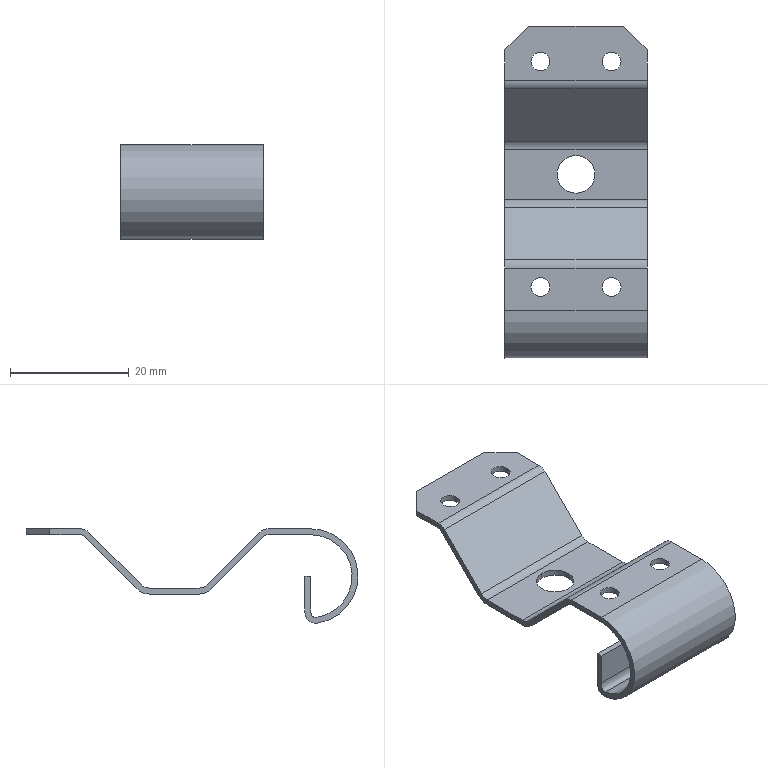Part | SolidWorks | features BaseBody 1 | 1 solid | 43 faces | box 24 x 56 x 15.934 mm | volume 1977 mm3 | cylinder 21 | plane 20 | spline 2 | commonest cylinder face diameters 3.2 x8 4 x5 2 x2 6 x2 6.35 x2 14 x1
STEP:
#1=CARTESIAN_POINT('',(4.4,-44.,0.));
#2=VERTEX_POINT('',#1);
#3=CARTESIAN_POINT('',(7.6,-44.,0.));
#4=VERTEX_POINT('',#3);
#5=CARTESIAN_POINT('',(6.,-44.,0.));
#6=DIRECTION('',(0.,0.,1.));
#7=DIRECTION('',(-1.,0.,0.));
#8=AXIS2_PLACEMENT_3D('',#5,#6,#7);
#9=CIRCLE('',#8,1.6);
#10=EDGE_CURVE('',#2,#4,#9,.T.);
#11=ORIENTED_EDGE('',*,*,#10,.T.);
#12=CARTESIAN_POINT('',(7.6,-44.,-1.));
#13=VERTEX_POINT('',#12);
#14=CARTESIAN_POINT('',(7.6,-44.,0.));
#15=DIRECTION('',(0.,0.,-1.));
#16=VECTOR('',#15,1000.);
#17=LINE('',#14,#16);
#18=EDGE_CURVE('',#4,#13,#17,.T.);
#19=ORIENTED_EDGE('',*,*,#18,.T.);
#20=CARTESIAN_POINT('',(4.4,-44.,-1.));
#21=VERTEX_POINT('',#20);
#22=CARTESIAN_POINT('',(6.,-44.,-1.));
#23=DIRECTION('',(0.,0.,-1.));
#24=DIRECTION('',(-1.,0.,0.));
#25=AXIS2_PLACEMENT_3D('',#22,#23,#24);
#26=CIRCLE('',#25,1.6);
#27=EDGE_CURVE('',#13,#21,#26,.T.);
#28=ORIENTED_EDGE('',*,*,#27,.T.);
#29=CARTESIAN_POINT('',(4.4,-44.,0.));
#30=DIRECTION('',(0.,0.,-1.));
#31=VECTOR('',#30,1000.);
#32=LINE('',#29,#31);
#33=EDGE_CURVE('',#2,#21,#32,.T.);
#34=ORIENTED_EDGE('',*,*,#33,.F.);
#35=EDGE_LOOP('',(#11,#19,#28,#34));
#36=FACE_OUTER_BOUND('',#35,.T.);
#37=CARTESIAN_POINT('',(6.,-44.,0.));
#38=DIRECTION('',(0.,0.,-1.));
#39=DIRECTION('',(-1.,0.,0.));
#40=AXIS2_PLACEMENT_3D('',#37,#38,#39);
#41=CYLINDRICAL_SURFACE('',#40,1.6);
#42=ADVANCED_FACE('',(#36),#41,.F.);
#43=CARTESIAN_POINT('',(16.4,-44.,0.));
#44=VERTEX_POINT('',#43);
#45=CARTESIAN_POINT('',(19.6,-44.,0.));
#46=VERTEX_POINT('',#45);
#47=CARTESIAN_POINT('',(18.,-44.,0.));
#48=DIRECTION('',(0.,0.,1.));
#49=DIRECTION('',(-1.,0.,0.));
#50=AXIS2_PLACEMENT_3D('',#47,#48,#49);
#51=CIRCLE('',#50,1.6);
#52=EDGE_CURVE('',#44,#46,#51,.T.);
#53=ORIENTED_EDGE('',*,*,#52,.T.);
#54=CARTESIAN_POINT('',(19.6,-44.,-1.));
#55=VERTEX_POINT('',#54);
#56=CARTESIAN_POINT('',(19.6,-44.,0.));
#57=DIRECTION('',(0.,0.,-1.));
#58=VECTOR('',#57,1000.);
#59=LINE('',#56,#58);
#60=EDGE_CURVE('',#46,#55,#59,.T.);
#61=ORIENTED_EDGE('',*,*,#60,.T.);
#62=CARTESIAN_POINT('',(16.4,-44.,-1.));
#63=VERTEX_POINT('',#62);
#64=CARTESIAN_POINT('',(18.,-44.,-1.));
#65=DIRECTION('',(0.,0.,-1.));
#66=DIRECTION('',(-1.,0.,0.));
#67=AXIS2_PLACEMENT_3D('',#64,#65,#66);
#68=CIRCLE('',#67,1.6);
#69=EDGE_CURVE('',#55,#63,#68,.T.);
#70=ORIENTED_EDGE('',*,*,#69,.T.);
#71=CARTESIAN_POINT('',(16.4,-44.,0.));
#72=DIRECTION('',(0.,0.,-1.));
#73=VECTOR('',#72,1000.);
#74=LINE('',#71,#73);
#75=EDGE_CURVE('',#44,#63,#74,.T.);
#76=ORIENTED_EDGE('',*,*,#75,.F.);
#77=EDGE_LOOP('',(#53,#61,#70,#76));
#78=FACE_OUTER_BOUND('',#77,.T.);
#79=CARTESIAN_POINT('',(18.,-44.,0.));
#80=DIRECTION('',(0.,0.,-1.));
#81=DIRECTION('',(-1.,0.,0.));
#82=AXIS2_PLACEMENT_3D('',#79,#80,#81);
#83=CYLINDRICAL_SURFACE('',#82,1.6);
#84=ADVANCED_FACE('',(#78),#83,.F.);
#85=CARTESIAN_POINT('',(16.4,-6.,0.));
#86=VERTEX_POINT('',#85);
#87=CARTESIAN_POINT('',(19.6,-6.,0.));
#88=VERTEX_POINT('',#87);
#89=CARTESIAN_POINT('',(18.,-6.,0.));
#90=DIRECTION('',(0.,0.,1.));
#91=DIRECTION('',(-1.,0.,0.));
#92=AXIS2_PLACEMENT_3D('',#89,#90,#91);
#93=CIRCLE('',#92,1.6);
#94=EDGE_CURVE('',#86,#88,#93,.T.);
#95=ORIENTED_EDGE('',*,*,#94,.T.);
#96=CARTESIAN_POINT('',(19.6,-6.,-1.));
#97=VERTEX_POINT('',#96);
#98=CARTESIAN_POINT('',(19.6,-6.,0.));
#99=DIRECTION('',(0.,0.,-1.));
#100=VECTOR('',#99,1000.);
#101=LINE('',#98,#100);
#102=EDGE_CURVE('',#88,#97,#101,.T.);
#103=ORIENTED_EDGE('',*,*,#102,.T.);
#104=CARTESIAN_POINT('',(16.4,-6.,-1.));
#105=VERTEX_POINT('',#104);
#106=CARTESIAN_POINT('',(18.,-6.,-1.));
#107=DIRECTION('',(0.,0.,-1.));
#108=DIRECTION('',(-1.,0.,0.));
#109=AXIS2_PLACEMENT_3D('',#106,#107,#108);
#110=CIRCLE('',#109,1.6);
#111=EDGE_CURVE('',#97,#105,#110,.T.);
#112=ORIENTED_EDGE('',*,*,#111,.T.);
#113=CARTESIAN_POINT('',(16.4,-6.,0.));
#114=DIRECTION('',(0.,0.,-1.));
#115=VECTOR('',#114,1000.);
#116=LINE('',#113,#115);
#117=EDGE_CURVE('',#86,#105,#116,.T.);
#118=ORIENTED_EDGE('',*,*,#117,.F.);
#119=EDGE_LOOP('',(#95,#103,#112,#118));
#120=FACE_OUTER_BOUND('',#119,.T.);
#121=CARTESIAN_POINT('',(18.,-6.,0.));
#122=DIRECTION('',(0.,0.,-1.));
#123=DIRECTION('',(-1.,0.,0.));
#124=AXIS2_PLACEMENT_3D('',#121,#122,#123);
#125=CYLINDRICAL_SURFACE('',#124,1.6);
#126=ADVANCED_FACE('',(#120),#125,.F.);
#127=CARTESIAN_POINT('',(4.4,-6.,0.));
#128=VERTEX_POINT('',#127);
#129=CARTESIAN_POINT('',(7.6,-6.,0.));
#130=VERTEX_POINT('',#129);
#131=CARTESIAN_POINT('',(6.,-6.,0.));
#132=DIRECTION('',(0.,0.,1.));
#133=DIRECTION('',(-1.,0.,0.));
#134=AXIS2_PLACEMENT_3D('',#131,#132,#133);
#135=CIRCLE('',#134,1.6);
#136=EDGE_CURVE('',#128,#130,#135,.T.);
#137=ORIENTED_EDGE('',*,*,#136,.T.);
#138=CARTESIAN_POINT('',(7.6,-6.,-1.));
#139=VERTEX_POINT('',#138);
#140=CARTESIAN_POINT('',(7.6,-6.,0.));
#141=DIRECTION('',(0.,0.,-1.));
#142=VECTOR('',#141,1000.);
#143=LINE('',#140,#142);
#144=EDGE_CURVE('',#130,#139,#143,.T.);
#145=ORIENTED_EDGE('',*,*,#144,.T.);
#146=CARTESIAN_POINT('',(4.4,-6.,-1.));
#147=VERTEX_POINT('',#146);
#148=CARTESIAN_POINT('',(6.,-6.,-1.));
#149=DIRECTION('',(0.,0.,-1.));
#150=DIRECTION('',(-1.,0.,0.));
#151=AXIS2_PLACEMENT_3D('',#148,#149,#150);
#152=CIRCLE('',#151,1.6);
#153=EDGE_CURVE('',#139,#147,#152,.T.);
#154=ORIENTED_EDGE('',*,*,#153,.T.);
#155=CARTESIAN_POINT('',(4.4,-6.,0.));
#156=DIRECTION('',(0.,0.,-1.));
#157=VECTOR('',#156,1000.);
#158=LINE('',#155,#157);
#159=EDGE_CURVE('',#128,#147,#158,.T.);
#160=ORIENTED_EDGE('',*,*,#159,.F.);
#161=EDGE_LOOP('',(#137,#145,#154,#160));
#162=FACE_OUTER_BOUND('',#161,.T.);
#163=CARTESIAN_POINT('',(6.,-6.,0.));
#164=DIRECTION('',(0.,0.,-1.));
#165=DIRECTION('',(-1.,0.,0.));
#166=AXIS2_PLACEMENT_3D('',#163,#164,#165);
#167=CYLINDRICAL_SURFACE('',#166,1.6);
#168=ADVANCED_FACE('',(#162),#167,.F.);
#169=CARTESIAN_POINT('',(12.,-21.825,-10.));
#170=VERTEX_POINT('',#169);
#171=CARTESIAN_POINT('',(12.,-28.175,-10.));
#172=VERTEX_POINT('',#171);
#173=CARTESIAN_POINT('',(12.,-25.,-10.));
#174=DIRECTION('',(0.,0.,1.));
#175=DIRECTION('',(0.,1.,0.));
#176=AXIS2_PLACEMENT_3D('',#173,#174,#175);
#177=CIRCLE('',#176,3.175);
#178=EDGE_CURVE('',#170,#172,#177,.T.);
#179=ORIENTED_EDGE('',*,*,#178,.T.);
#180=CARTESIAN_POINT('',(12.,-28.175,-11.));
#181=VERTEX_POINT('',#180);
#182=CARTESIAN_POINT('',(12.,-28.175,-10.));
#183=DIRECTION('',(0.,0.,-1.));
#184=VECTOR('',#183,1000.);
#185=LINE('',#182,#184);
#186=EDGE_CURVE('',#172,#181,#185,.T.);
#187=ORIENTED_EDGE('',*,*,#186,.T.);
#188=CARTESIAN_POINT('',(12.,-21.825,-11.));
#189=VERTEX_POINT('',#188);
#190=CARTESIAN_POINT('',(12.,-25.,-11.));
#191=DIRECTION('',(0.,0.,-1.));
#192=DIRECTION('',(0.,1.,0.));
#193=AXIS2_PLACEMENT_3D('',#190,#191,#192);
#194=CIRCLE('',#193,3.175);
#195=EDGE_CURVE('',#181,#189,#194,.T.);
#196=ORIENTED_EDGE('',*,*,#195,.T.);
#197=CARTESIAN_POINT('',(12.,-21.825,-10.));
#198=DIRECTION('',(0.,0.,-1.));
#199=VECTOR('',#198,1000.);
#200=LINE('',#197,#199);
#201=EDGE_CURVE('',#170,#189,#200,.T.);
#202=ORIENTED_EDGE('',*,*,#201,.F.);
#203=EDGE_LOOP('',(#179,#187,#196,#202));
#204=FACE_OUTER_BOUND('',#203,.T.);
#205=CARTESIAN_POINT('',(12.,-25.,-10.));
#206=DIRECTION('',(0.,0.,-1.));
#207=DIRECTION('',(0.,1.,0.));
#208=AXIS2_PLACEMENT_3D('',#205,#206,#207);
#209=CYLINDRICAL_SURFACE('',#208,3.175);
#210=ADVANCED_FACE('',(#204),#209,.F.);
#211=ORIENTED_EDGE('',*,*,#18,.F.);
#212=CARTESIAN_POINT('',(6.,-44.,0.));
#213=DIRECTION('',(0.,0.,1.));
#214=DIRECTION('',(-1.,0.,0.));
#215=AXIS2_PLACEMENT_3D('',#212,#213,#214);
#216=CIRCLE('',#215,1.6);
#217=EDGE_CURVE('',#4,#2,#216,.T.);
#218=ORIENTED_EDGE('',*,*,#217,.T.);
#219=ORIENTED_EDGE('',*,*,#33,.T.);
#220=CARTESIAN_POINT('',(6.,-44.,-1.));
#221=DIRECTION('',(0.,0.,-1.));
#222=DIRECTION('',(-1.,0.,0.));
#223=AXIS2_PLACEMENT_3D('',#220,#221,#222);
#224=CIRCLE('',#223,1.6);
#225=EDGE_CURVE('',#21,#13,#224,.T.);
#226=ORIENTED_EDGE('',*,*,#225,.T.);
#227=EDGE_LOOP('',(#211,#218,#219,#226));
#228=FACE_OUTER_BOUND('',#227,.T.);
#229=CARTESIAN_POINT('',(6.,-44.,0.));
#230=DIRECTION('',(0.,0.,-1.));
#231=DIRECTION('',(-1.,0.,0.));
#232=AXIS2_PLACEMENT_3D('',#229,#230,#231);
#233=CYLINDRICAL_SURFACE('',#232,1.6);
#234=ADVANCED_FACE('',(#228),#233,.F.);
#235=CARTESIAN_POINT('',(18.,-44.,-1.));
#236=DIRECTION('',(0.,0.,-1.));
#237=DIRECTION('',(-1.,0.,0.));
#238=AXIS2_PLACEMENT_3D('',#235,#236,#237);
#239=CIRCLE('',#238,1.6);
#240=EDGE_CURVE('',#63,#55,#239,.T.);
#241=ORIENTED_EDGE('',*,*,#240,.F.);
#242=ORIENTED_EDGE('',*,*,#69,.F.);
#243=EDGE_LOOP('',(#241,#242));
#244=FACE_BOUND('',#243,.T.);
#245=ORIENTED_EDGE('',*,*,#225,.F.);
#246=ORIENTED_EDGE('',*,*,#27,.F.);
#247=EDGE_LOOP('',(#245,#246));
#248=FACE_BOUND('',#247,.T.);
#249=CARTESIAN_POINT('',(24.,-40.828,-1.));
#250=VERTEX_POINT('',#249);
#251=CARTESIAN_POINT('',(0.,-40.828,-1.));
#252=VERTEX_POINT('',#251);
#253=CARTESIAN_POINT('',(12.,-40.828,-1.));
#254=DIRECTION('',(-1.,0.,0.));
#255=VECTOR('',#254,1000.);
#256=LINE('',#253,#255);
#257=EDGE_CURVE('',#250,#252,#256,.T.);
#258=ORIENTED_EDGE('',*,*,#257,.F.);
#259=CARTESIAN_POINT('',(24.,-48.,-1.));
#260=VERTEX_POINT('',#259);
#261=CARTESIAN_POINT('',(24.,-44.414,-1.));
#262=DIRECTION('',(0.,1.,0.));
#263=VECTOR('',#262,1000.);
#264=LINE('',#261,#263);
#265=EDGE_CURVE('',#260,#250,#264,.T.);
#266=ORIENTED_EDGE('',*,*,#265,.F.);
#267=CARTESIAN_POINT('',(0.,-48.,-1.));
#268=VERTEX_POINT('',#267);
#269=CARTESIAN_POINT('',(12.,-48.,-1.));
#270=DIRECTION('',(1.,0.,0.));
#271=VECTOR('',#270,1000.);
#272=LINE('',#269,#271);
#273=EDGE_CURVE('',#268,#260,#272,.T.);
#274=ORIENTED_EDGE('',*,*,#273,.F.);
#275=CARTESIAN_POINT('',(0.,-44.414,-1.));
#276=DIRECTION('',(0.,-1.,0.));
#277=VECTOR('',#276,1000.);
#278=LINE('',#275,#277);
#279=EDGE_CURVE('',#252,#268,#278,.T.);
#280=ORIENTED_EDGE('',*,*,#279,.F.);
#281=EDGE_LOOP('',(#258,#266,#274,#280));
#282=FACE_OUTER_BOUND('',#281,.T.);
#283=CARTESIAN_POINT('',(0.,-40.828,-1.));
#284=DIRECTION('',(0.,0.,1.));
#285=DIRECTION('',(0.,-1.,0.));
#286=AXIS2_PLACEMENT_3D('',#283,#284,#285);
#287=PLANE('',#286);
#288=ADVANCED_FACE('',(#244,#248,#282),#287,.F.);
#289=ORIENTED_EDGE('',*,*,#52,.F.);
#290=CARTESIAN_POINT('',(18.,-44.,0.));
#291=DIRECTION('',(0.,0.,1.));
#292=DIRECTION('',(-1.,0.,0.));
#293=AXIS2_PLACEMENT_3D('',#290,#291,#292);
#294=CIRCLE('',#293,1.6);
#295=EDGE_CURVE('',#46,#44,#294,.T.);
#296=ORIENTED_EDGE('',*,*,#295,.F.);
#297=EDGE_LOOP('',(#289,#296));
#298=FACE_BOUND('',#297,.T.);
#299=ORIENTED_EDGE('',*,*,#10,.F.);
#300=ORIENTED_EDGE('',*,*,#217,.F.);
#301=EDGE_LOOP('',(#299,#300));
#302=FACE_BOUND('',#301,.T.);
#303=CARTESIAN_POINT('',(24.,-48.,0.));
#304=VERTEX_POINT('',#303);
#305=CARTESIAN_POINT('',(0.,-48.,0.));
#306=VERTEX_POINT('',#305);
#307=CARTESIAN_POINT('',(12.,-48.,0.));
#308=DIRECTION('',(-1.,0.,0.));
#309=VECTOR('',#308,1000.);
#310=LINE('',#307,#309);
#311=EDGE_CURVE('',#304,#306,#310,.T.);
#312=ORIENTED_EDGE('',*,*,#311,.F.);
#313=CARTESIAN_POINT('',(24.,-40.828,0.));
#314=VERTEX_POINT('',#313);
#315=CARTESIAN_POINT('',(24.,-44.414,0.));
#316=DIRECTION('',(0.,-1.,0.));
#317=VECTOR('',#316,1000.);
#318=LINE('',#315,#317);
#319=EDGE_CURVE('',#314,#304,#318,.T.);
#320=ORIENTED_EDGE('',*,*,#319,.F.);
#321=CARTESIAN_POINT('',(0.,-40.828,0.));
#322=VERTEX_POINT('',#321);
#323=CARTESIAN_POINT('',(12.,-40.828,0.));
#324=DIRECTION('',(1.,0.,0.));
#325=VECTOR('',#324,1000.);
#326=LINE('',#323,#325);
#327=EDGE_CURVE('',#322,#314,#326,.T.);
#328=ORIENTED_EDGE('',*,*,#327,.F.);
#329=CARTESIAN_POINT('',(0.,-44.414,0.));
#330=DIRECTION('',(0.,1.,0.));
#331=VECTOR('',#330,1000.);
#332=LINE('',#329,#331);
#333=EDGE_CURVE('',#306,#322,#332,.T.);
#334=ORIENTED_EDGE('',*,*,#333,.F.);
#335=EDGE_LOOP('',(#312,#320,#328,#334));
#336=FACE_OUTER_BOUND('',#335,.T.);
#337=CARTESIAN_POINT('',(0.,-48.,0.));
#338=DIRECTION('',(0.,0.,-1.));
#339=DIRECTION('',(0.,1.,0.));
#340=AXIS2_PLACEMENT_3D('',#337,#338,#339);
#341=PLANE('',#340);
#342=ADVANCED_FACE('',(#298,#302,#336),#341,.F.);
#343=ORIENTED_EDGE('',*,*,#60,.F.);
#344=ORIENTED_EDGE('',*,*,#295,.T.);
#345=ORIENTED_EDGE('',*,*,#75,.T.);
#346=ORIENTED_EDGE('',*,*,#240,.T.);
#347=EDGE_LOOP('',(#343,#344,#345,#346));
#348=FACE_OUTER_BOUND('',#347,.T.);
#349=CARTESIAN_POINT('',(18.,-44.,0.));
#350=DIRECTION('',(0.,0.,-1.));
#351=DIRECTION('',(-1.,0.,0.));
#352=AXIS2_PLACEMENT_3D('',#349,#350,#351);
#353=CYLINDRICAL_SURFACE('',#352,1.6);
#354=ADVANCED_FACE('',(#348),#353,.F.);
#355=CARTESIAN_POINT('',(0.,-4.,0.));
#356=VERTEX_POINT('',#355);
#357=CARTESIAN_POINT('',(0.,-4.,-1.));
#358=VERTEX_POINT('',#357);
#359=CARTESIAN_POINT('',(0.,-4.,-0.5));
#360=DIRECTION('',(0.,0.,-1.));
#361=VECTOR('',#360,1000.);
#362=LINE('',#359,#361);
#363=EDGE_CURVE('',#356,#358,#362,.T.);
#364=ORIENTED_EDGE('',*,*,#363,.T.);
#365=CARTESIAN_POINT('',(0.,-9.172,-1.));
#366=VERTEX_POINT('',#365);
#367=CARTESIAN_POINT('',(0.,-30.156,-1.));
#368=DIRECTION('',(0.,1.,0.));
#369=VECTOR('',#368,1000.);
#370=LINE('',#367,#369);
#371=EDGE_CURVE('',#366,#358,#370,.T.);
#372=ORIENTED_EDGE('',*,*,#371,.F.);
#373=CARTESIAN_POINT('',(0.,-9.879,-1.293));
#374=VERTEX_POINT('',#373);
#375=CARTESIAN_POINT('',(0.,-9.172,-2.));
#376=DIRECTION('',(-1.,0.,0.));
#377=DIRECTION('',(0.,0.,1.));
#378=AXIS2_PLACEMENT_3D('',#375,#376,#377);
#379=CIRCLE('',#378,1.);
#380=EDGE_CURVE('',#374,#366,#379,.T.);
#381=ORIENTED_EDGE('',*,*,#380,.F.);
#382=CARTESIAN_POINT('',(0.,-18.707,-10.121));
#383=VERTEX_POINT('',#382);
#384=CARTESIAN_POINT('',(0.,-9.879,-1.293));
#385=DIRECTION('',(0.,0.7071,0.7071));
#386=VECTOR('',#385,1000.);
#387=LINE('',#384,#386);
#388=EDGE_CURVE('',#383,#374,#387,.T.);
#389=ORIENTED_EDGE('',*,*,#388,.F.);
#390=CARTESIAN_POINT('',(0.,-20.828,-11.));
#391=VERTEX_POINT('',#390);
#392=CARTESIAN_POINT('',(0.,-20.828,-8.));
#393=DIRECTION('',(1.,0.,0.));
#394=DIRECTION('',(0.,0.,1.));
#395=AXIS2_PLACEMENT_3D('',#392,#393,#394);
#396=CIRCLE('',#395,3.);
#397=EDGE_CURVE('',#391,#383,#396,.T.);
#398=ORIENTED_EDGE('',*,*,#397,.F.);
#399=CARTESIAN_POINT('',(0.,-29.172,-11.));
#400=VERTEX_POINT('',#399);
#401=CARTESIAN_POINT('',(0.,-30.156,-11.));
#402=DIRECTION('',(0.,1.,0.));
#403=VECTOR('',#402,1000.);
#404=LINE('',#401,#403);
#405=EDGE_CURVE('',#400,#391,#404,.T.);
#406=ORIENTED_EDGE('',*,*,#405,.F.);
#407=CARTESIAN_POINT('',(0.,-31.293,-10.121));
#408=VERTEX_POINT('',#407);
#409=CARTESIAN_POINT('',(0.,-29.172,-8.));
#410=DIRECTION('',(1.,0.,0.));
#411=DIRECTION('',(0.,0.,1.));
#412=AXIS2_PLACEMENT_3D('',#409,#410,#411);
#413=CIRCLE('',#412,3.);
#414=EDGE_CURVE('',#408,#400,#413,.T.);
#415=ORIENTED_EDGE('',*,*,#414,.F.);
#416=CARTESIAN_POINT('',(0.,-40.121,-1.293));
#417=VERTEX_POINT('',#416);
#418=CARTESIAN_POINT('',(0.,-31.293,-10.121));
#419=DIRECTION('',(0.,0.7071,-0.7071));
#420=VECTOR('',#419,1000.);
#421=LINE('',#418,#420);
#422=EDGE_CURVE('',#417,#408,#421,.T.);
#423=ORIENTED_EDGE('',*,*,#422,.F.);
#424=CARTESIAN_POINT('',(0.,-40.828,-2.));
#425=DIRECTION('',(-1.,0.,0.));
#426=DIRECTION('',(0.,0.,1.));
#427=AXIS2_PLACEMENT_3D('',#424,#425,#426);
#428=CIRCLE('',#427,1.);
#429=EDGE_CURVE('',#252,#417,#428,.T.);
#430=ORIENTED_EDGE('',*,*,#429,.F.);
#431=ORIENTED_EDGE('',*,*,#279,.T.);
#432=CARTESIAN_POINT('',(0.,-49.061,-14.919));
#433=VERTEX_POINT('',#432);
#434=CARTESIAN_POINT('',(0.,-48.,-8.));
#435=DIRECTION('',(-1.,0.,0.));
#436=DIRECTION('',(0.,0.,1.));
#437=AXIS2_PLACEMENT_3D('',#434,#435,#436);
#438=CIRCLE('',#437,7.);
#439=EDGE_CURVE('',#433,#268,#438,.T.);
#440=ORIENTED_EDGE('',*,*,#439,.F.);
#441=CARTESIAN_POINT('',(0.,-48.,-13.525));
#442=VERTEX_POINT('',#441);
#443=CARTESIAN_POINT('',(0.,-48.,-13.525));
#444=CARTESIAN_POINT('',(0.,-48.,-13.685));
#445=CARTESIAN_POINT('',(0.,-48.019,-14.03));
#446=CARTESIAN_POINT('',(0.,-48.12,-14.503));
#447=CARTESIAN_POINT('',(0.,-48.264,-14.743));
#448=CARTESIAN_POINT('',(0.,-48.382,-14.839));
#449=CARTESIAN_POINT('',(0.,-48.506,-14.898));
#450=CARTESIAN_POINT('',(0.,-48.706,-14.941));
#451=CARTESIAN_POINT('',(0.,-48.953,-14.932));
#452=CARTESIAN_POINT('',(0.,-49.061,-14.919));
#453=B_SPLINE_CURVE_WITH_KNOTS('',3,(#443,#444,#445,#446,#447,#448,#449,#450,#451,#452),.UNSPECIFIED.,.F.,.F.,(4,1,1,1,1,1,1,4),(0.,0.0002613,0.0005226,0.001045,0.001306,0.001568,0.001829,0.00209),.UNSPECIFIED.);
#454=EDGE_CURVE('',#442,#433,#453,.T.);
#455=ORIENTED_EDGE('',*,*,#454,.F.);
#456=CARTESIAN_POINT('',(0.,-48.,-8.011));
#457=VERTEX_POINT('',#456);
#458=CARTESIAN_POINT('',(0.,-48.,-8.021));
#459=DIRECTION('',(0.,0.,-1.));
#460=VECTOR('',#459,1000.);
#461=LINE('',#458,#460);
#462=EDGE_CURVE('',#457,#442,#461,.T.);
#463=ORIENTED_EDGE('',*,*,#462,.F.);
#464=CARTESIAN_POINT('',(0.,-47.,-8.011));
#465=VERTEX_POINT('',#464);
#466=CARTESIAN_POINT('',(0.,-47.5,-8.011));
#467=DIRECTION('',(0.,1.,0.));
#468=VECTOR('',#467,1000.);
#469=LINE('',#466,#468);
#470=EDGE_CURVE('',#457,#465,#469,.T.);
#471=ORIENTED_EDGE('',*,*,#470,.T.);
#472=CARTESIAN_POINT('',(0.,-47.,-13.525));
#473=VERTEX_POINT('',#472);
#474=CARTESIAN_POINT('',(0.,-47.,-8.021));
#475=DIRECTION('',(0.,0.,1.));
#476=VECTOR('',#475,1000.);
#477=LINE('',#474,#476);
#478=EDGE_CURVE('',#473,#465,#477,.T.);
#479=ORIENTED_EDGE('',*,*,#478,.F.);
#480=CARTESIAN_POINT('',(0.,-49.198,-15.91));
#481=VERTEX_POINT('',#480);
#482=CARTESIAN_POINT('',(0.,-49.198,-15.91));
#483=CARTESIAN_POINT('',(0.,-47.739,-16.093));
#484=CARTESIAN_POINT('',(0.,-47.,-15.237));
#485=CARTESIAN_POINT('',(0.,-47.,-13.525));
#486=B_SPLINE_CURVE_WITH_KNOTS('',3,(#482,#483,#484,#485),.UNSPECIFIED.,.F.,.F.,(4,4),(0.,0.003798),.UNSPECIFIED.);
#487=EDGE_CURVE('',#481,#473,#486,.T.);
#488=ORIENTED_EDGE('',*,*,#487,.F.);
#489=CARTESIAN_POINT('',(0.,-48.,-8.));
#490=DIRECTION('',(1.,0.,0.));
#491=DIRECTION('',(0.,0.,1.));
#492=AXIS2_PLACEMENT_3D('',#489,#490,#491);
#493=CIRCLE('',#492,8.);
#494=EDGE_CURVE('',#306,#481,#493,.T.);
#495=ORIENTED_EDGE('',*,*,#494,.F.);
#496=ORIENTED_EDGE('',*,*,#333,.T.);
#497=CARTESIAN_POINT('',(0.,-39.414,-0.5858));
#498=VERTEX_POINT('',#497);
#499=CARTESIAN_POINT('',(0.,-40.828,-2.));
#500=DIRECTION('',(1.,0.,0.));
#501=DIRECTION('',(0.,0.,1.));
#502=AXIS2_PLACEMENT_3D('',#499,#500,#501);
#503=CIRCLE('',#502,2.);
#504=EDGE_CURVE('',#498,#322,#503,.T.);
#505=ORIENTED_EDGE('',*,*,#504,.F.);
#506=CARTESIAN_POINT('',(0.,-30.586,-9.414));
#507=VERTEX_POINT('',#506);
#508=CARTESIAN_POINT('',(0.,-39.414,-0.5858));
#509=DIRECTION('',(0.,-0.7071,0.7071));
#510=VECTOR('',#509,1000.);
#511=LINE('',#508,#510);
#512=EDGE_CURVE('',#507,#498,#511,.T.);
#513=ORIENTED_EDGE('',*,*,#512,.F.);
#514=CARTESIAN_POINT('',(0.,-29.172,-10.));
#515=VERTEX_POINT('',#514);
#516=CARTESIAN_POINT('',(0.,-29.172,-8.));
#517=DIRECTION('',(-1.,0.,0.));
#518=DIRECTION('',(0.,0.,1.));
#519=AXIS2_PLACEMENT_3D('',#516,#517,#518);
#520=CIRCLE('',#519,2.);
#521=EDGE_CURVE('',#515,#507,#520,.T.);
#522=ORIENTED_EDGE('',*,*,#521,.F.);
#523=CARTESIAN_POINT('',(0.,-20.828,-10.));
#524=VERTEX_POINT('',#523);
#525=CARTESIAN_POINT('',(0.,-30.156,-10.));
#526=DIRECTION('',(0.,-1.,0.));
#527=VECTOR('',#526,1000.);
#528=LINE('',#525,#527);
#529=EDGE_CURVE('',#524,#515,#528,.T.);
#530=ORIENTED_EDGE('',*,*,#529,.F.);
#531=CARTESIAN_POINT('',(0.,-19.414,-9.414));
#532=VERTEX_POINT('',#531);
#533=CARTESIAN_POINT('',(0.,-20.828,-8.));
#534=DIRECTION('',(-1.,0.,0.));
#535=DIRECTION('',(0.,0.,1.));
#536=AXIS2_PLACEMENT_3D('',#533,#534,#535);
#537=CIRCLE('',#536,2.);
#538=EDGE_CURVE('',#532,#524,#537,.T.);
#539=ORIENTED_EDGE('',*,*,#538,.F.);
#540=CARTESIAN_POINT('',(0.,-10.586,-0.5858));
#541=VERTEX_POINT('',#540);
#542=CARTESIAN_POINT('',(0.,-19.414,-9.414));
#543=DIRECTION('',(0.,-0.7071,-0.7071));
#544=VECTOR('',#543,1000.);
#545=LINE('',#542,#544);
#546=EDGE_CURVE('',#541,#532,#545,.T.);
#547=ORIENTED_EDGE('',*,*,#546,.F.);
#548=CARTESIAN_POINT('',(0.,-9.172,0.));
#549=VERTEX_POINT('',#548);
#550=CARTESIAN_POINT('',(0.,-9.172,-2.));
#551=DIRECTION('',(-1.,0.,0.));
#552=DIRECTION('',(0.,0.,1.));
#553=AXIS2_PLACEMENT_3D('',#550,#551,#552);
#554=CIRCLE('',#553,2.);
#555=EDGE_CURVE('',#541,#549,#554,.T.);
#556=ORIENTED_EDGE('',*,*,#555,.T.);
#557=CARTESIAN_POINT('',(0.,-30.156,0.));
#558=DIRECTION('',(0.,-1.,0.));
#559=VECTOR('',#558,1000.);
#560=LINE('',#557,#559);
#561=EDGE_CURVE('',#356,#549,#560,.T.);
#562=ORIENTED_EDGE('',*,*,#561,.F.);
#563=EDGE_LOOP('',(#364,#372,#381,#389,#398,#406,#415,#423,#430,#431,#440,#455,#463,#471,#479,#488,#495,#496,#505,#513,#522,#530,#539,#547,#556,#562));
#564=FACE_OUTER_BOUND('',#563,.T.);
#565=CARTESIAN_POINT('',(0.,-56.312,0.));
#566=DIRECTION('',(1.,0.,0.));
#567=DIRECTION('',(0.,0.,-1.));
#568=AXIS2_PLACEMENT_3D('',#565,#566,#567);
#569=PLANE('',#568);
#570=ADVANCED_FACE('',(#564),#569,.F.);
#571=CARTESIAN_POINT('',(24.,-40.121,-1.293));
#572=VERTEX_POINT('',#571);
#573=CARTESIAN_POINT('',(24.,-40.828,-2.));
#574=DIRECTION('',(1.,0.,0.));
#575=DIRECTION('',(0.,0.,1.));
#576=AXIS2_PLACEMENT_3D('',#573,#574,#575);
#577=CIRCLE('',#576,1.);
#578=EDGE_CURVE('',#572,#250,#577,.T.);
#579=ORIENTED_EDGE('',*,*,#578,.T.);
#580=ORIENTED_EDGE('',*,*,#257,.T.);
#581=ORIENTED_EDGE('',*,*,#429,.T.);
#582=CARTESIAN_POINT('',(12.,-40.121,-1.293));
#583=DIRECTION('',(1.,0.,0.));
#584=VECTOR('',#583,1000.);
#585=LINE('',#582,#584);
#586=EDGE_CURVE('',#417,#572,#585,.T.);
#587=ORIENTED_EDGE('',*,*,#586,.T.);
#588=EDGE_LOOP('',(#579,#580,#581,#587));
#589=FACE_OUTER_BOUND('',#588,.T.);
#590=CARTESIAN_POINT('',(24.,-40.828,-2.));
#591=DIRECTION('',(-1.,0.,0.));
#592=DIRECTION('',(0.,0.,1.));
#593=AXIS2_PLACEMENT_3D('',#590,#591,#592);
#594=CYLINDRICAL_SURFACE('',#593,1.);
#595=ADVANCED_FACE('',(#589),#594,.F.);
#596=CARTESIAN_POINT('',(24.,-49.198,-15.91));
#597=VERTEX_POINT('',#596);
#598=CARTESIAN_POINT('',(24.,-47.,-13.525));
#599=VERTEX_POINT('',#598);
#600=CARTESIAN_POINT('',(24.,-49.198,-15.91));
#601=CARTESIAN_POINT('',(24.,-47.739,-16.093));
#602=CARTESIAN_POINT('',(24.,-47.,-15.237));
#603=CARTESIAN_POINT('',(24.,-47.,-13.525));
#604=B_SPLINE_CURVE_WITH_KNOTS('',3,(#600,#601,#602,#603),.UNSPECIFIED.,.F.,.F.,(4,4),(0.,0.003798),.UNSPECIFIED.);
#605=EDGE_CURVE('',#597,#599,#604,.T.);
#606=ORIENTED_EDGE('',*,*,#605,.T.);
#607=CARTESIAN_POINT('',(24.,-47.,-11.011));
#608=VERTEX_POINT('',#607);
#609=CARTESIAN_POINT('',(24.,-47.,-8.021));
#610=DIRECTION('',(0.,0.,1.));
#611=VECTOR('',#610,1000.);
#612=LINE('',#609,#611);
#613=EDGE_CURVE('',#599,#608,#612,.T.);
#614=ORIENTED_EDGE('',*,*,#613,.T.);
#615=CARTESIAN_POINT('',(24.,-48.,-11.011));
#616=VERTEX_POINT('',#615);
#617=CARTESIAN_POINT('',(24.,-47.5,-11.011));
#618=DIRECTION('',(0.,-1.,0.));
#619=VECTOR('',#618,1000.);
#620=LINE('',#617,#619);
#621=EDGE_CURVE('',#608,#616,#620,.T.);
#622=ORIENTED_EDGE('',*,*,#621,.T.);
#623=CARTESIAN_POINT('',(24.,-48.,-13.525));
#624=VERTEX_POINT('',#623);
#625=CARTESIAN_POINT('',(24.,-48.,-8.021));
#626=DIRECTION('',(0.,0.,-1.));
#627=VECTOR('',#626,1000.);
#628=LINE('',#625,#627);
#629=EDGE_CURVE('',#616,#624,#628,.T.);
#630=ORIENTED_EDGE('',*,*,#629,.T.);
#631=CARTESIAN_POINT('',(24.,-49.061,-14.919));
#632=VERTEX_POINT('',#631);
#633=CARTESIAN_POINT('',(24.,-48.,-13.525));
#634=CARTESIAN_POINT('',(24.,-48.,-13.685));
#635=CARTESIAN_POINT('',(24.,-48.019,-14.03));
#636=CARTESIAN_POINT('',(24.,-48.12,-14.503));
#637=CARTESIAN_POINT('',(24.,-48.264,-14.743));
#638=CARTESIAN_POINT('',(24.,-48.382,-14.839));
#639=CARTESIAN_POINT('',(24.,-48.506,-14.898));
#640=CARTESIAN_POINT('',(24.,-48.706,-14.941));
#641=CARTESIAN_POINT('',(24.,-48.953,-14.932));
#642=CARTESIAN_POINT('',(24.,-49.061,-14.919));
#643=B_SPLINE_CURVE_WITH_KNOTS('',3,(#633,#634,#635,#636,#637,#638,#639,#640,#641,#642),.UNSPECIFIED.,.F.,.F.,(4,1,1,1,1,1,1,4),(0.,0.0002613,0.0005226,0.001045,0.001306,0.001568,0.001829,0.00209),.UNSPECIFIED.);
#644=EDGE_CURVE('',#624,#632,#643,.T.);
#645=ORIENTED_EDGE('',*,*,#644,.T.);
#646=CARTESIAN_POINT('',(24.,-48.,-8.));
#647=DIRECTION('',(-1.,0.,0.));
#648=DIRECTION('',(0.,0.,1.));
#649=AXIS2_PLACEMENT_3D('',#646,#647,#648);
#650=CIRCLE('',#649,7.);
#651=EDGE_CURVE('',#632,#260,#650,.T.);
#652=ORIENTED_EDGE('',*,*,#651,.T.);
#653=ORIENTED_EDGE('',*,*,#265,.T.);
#654=ORIENTED_EDGE('',*,*,#578,.F.);
#655=CARTESIAN_POINT('',(24.,-31.293,-10.121));
#656=VERTEX_POINT('',#655);
#657=CARTESIAN_POINT('',(24.,-40.121,-1.293));
#658=DIRECTION('',(0.,0.7071,-0.7071));
#659=VECTOR('',#658,1000.);
#660=LINE('',#657,#659);
#661=EDGE_CURVE('',#572,#656,#660,.T.);
#662=ORIENTED_EDGE('',*,*,#661,.T.);
#663=CARTESIAN_POINT('',(24.,-29.172,-11.));
#664=VERTEX_POINT('',#663);
#665=CARTESIAN_POINT('',(24.,-29.172,-8.));
#666=DIRECTION('',(1.,0.,0.));
#667=DIRECTION('',(0.,0.,1.));
#668=AXIS2_PLACEMENT_3D('',#665,#666,#667);
#669=CIRCLE('',#668,3.);
#670=EDGE_CURVE('',#656,#664,#669,.T.);
#671=ORIENTED_EDGE('',*,*,#670,.T.);
#672=CARTESIAN_POINT('',(24.,-20.828,-11.));
#673=VERTEX_POINT('',#672);
#674=CARTESIAN_POINT('',(24.,-30.156,-11.));
#675=DIRECTION('',(0.,1.,0.));
#676=VECTOR('',#675,1000.);
#677=LINE('',#674,#676);
#678=EDGE_CURVE('',#664,#673,#677,.T.);
#679=ORIENTED_EDGE('',*,*,#678,.T.);
#680=CARTESIAN_POINT('',(24.,-18.707,-10.121));
#681=VERTEX_POINT('',#680);
#682=CARTESIAN_POINT('',(24.,-20.828,-8.));
#683=DIRECTION('',(1.,0.,0.));
#684=DIRECTION('',(0.,0.,1.));
#685=AXIS2_PLACEMENT_3D('',#682,#683,#684);
#686=CIRCLE('',#685,3.);
#687=EDGE_CURVE('',#673,#681,#686,.T.);
#688=ORIENTED_EDGE('',*,*,#687,.T.);
#689=CARTESIAN_POINT('',(24.,-9.879,-1.293));
#690=VERTEX_POINT('',#689);
#691=CARTESIAN_POINT('',(24.,-18.707,-10.121));
#692=DIRECTION('',(0.,0.7071,0.7071));
#693=VECTOR('',#692,1000.);
#694=LINE('',#691,#693);
#695=EDGE_CURVE('',#681,#690,#694,.T.);
#696=ORIENTED_EDGE('',*,*,#695,.T.);
#697=CARTESIAN_POINT('',(24.,-9.172,-1.));
#698=VERTEX_POINT('',#697);
#699=CARTESIAN_POINT('',(24.,-9.172,-2.));
#700=DIRECTION('',(1.,0.,0.));
#701=DIRECTION('',(0.,0.,1.));
#702=AXIS2_PLACEMENT_3D('',#699,#700,#701);
#703=CIRCLE('',#702,1.);
#704=EDGE_CURVE('',#698,#690,#703,.T.);
#705=ORIENTED_EDGE('',*,*,#704,.F.);
#706=CARTESIAN_POINT('',(24.,-4.,-1.));
#707=VERTEX_POINT('',#706);
#708=CARTESIAN_POINT('',(24.,-30.156,-1.));
#709=DIRECTION('',(0.,1.,0.));
#710=VECTOR('',#709,1000.);
#711=LINE('',#708,#710);
#712=EDGE_CURVE('',#698,#707,#711,.T.);
#713=ORIENTED_EDGE('',*,*,#712,.T.);
#714=CARTESIAN_POINT('',(24.,-4.,0.));
#715=VERTEX_POINT('',#714);
#716=CARTESIAN_POINT('',(24.,-4.,-0.5));
#717=DIRECTION('',(0.,0.,-1.));
#718=VECTOR('',#717,1000.);
#719=LINE('',#716,#718);
#720=EDGE_CURVE('',#715,#707,#719,.T.);
#721=ORIENTED_EDGE('',*,*,#720,.F.);
#722=CARTESIAN_POINT('',(24.,-9.172,0.));
#723=VERTEX_POINT('',#722);
#724=CARTESIAN_POINT('',(24.,-30.156,0.));
#725=DIRECTION('',(0.,-1.,0.));
#726=VECTOR('',#725,1000.);
#727=LINE('',#724,#726);
#728=EDGE_CURVE('',#715,#723,#727,.T.);
#729=ORIENTED_EDGE('',*,*,#728,.T.);
#730=CARTESIAN_POINT('',(24.,-10.586,-0.5858));
#731=VERTEX_POINT('',#730);
#732=CARTESIAN_POINT('',(24.,-9.172,-2.));
#733=DIRECTION('',(1.,0.,0.));
#734=DIRECTION('',(0.,0.,1.));
#735=AXIS2_PLACEMENT_3D('',#732,#733,#734);
#736=CIRCLE('',#735,2.);
#737=EDGE_CURVE('',#723,#731,#736,.T.);
#738=ORIENTED_EDGE('',*,*,#737,.T.);
#739=CARTESIAN_POINT('',(24.,-19.414,-9.414));
#740=VERTEX_POINT('',#739);
#741=CARTESIAN_POINT('',(24.,-10.586,-0.5858));
#742=DIRECTION('',(0.,-0.7071,-0.7071));
#743=VECTOR('',#742,1000.);
#744=LINE('',#741,#743);
#745=EDGE_CURVE('',#731,#740,#744,.T.);
#746=ORIENTED_EDGE('',*,*,#745,.T.);
#747=CARTESIAN_POINT('',(24.,-20.828,-10.));
#748=VERTEX_POINT('',#747);
#749=CARTESIAN_POINT('',(24.,-20.828,-8.));
#750=DIRECTION('',(1.,0.,0.));
#751=DIRECTION('',(0.,0.,1.));
#752=AXIS2_PLACEMENT_3D('',#749,#750,#751);
#753=CIRCLE('',#752,2.);
#754=EDGE_CURVE('',#748,#740,#753,.T.);
#755=ORIENTED_EDGE('',*,*,#754,.F.);
#756=CARTESIAN_POINT('',(24.,-29.172,-10.));
#757=VERTEX_POINT('',#756);
#758=CARTESIAN_POINT('',(24.,-30.156,-10.));
#759=DIRECTION('',(0.,-1.,0.));
#760=VECTOR('',#759,1000.);
#761=LINE('',#758,#760);
#762=EDGE_CURVE('',#748,#757,#761,.T.);
#763=ORIENTED_EDGE('',*,*,#762,.T.);
#764=CARTESIAN_POINT('',(24.,-30.586,-9.414));
#765=VERTEX_POINT('',#764);
#766=CARTESIAN_POINT('',(24.,-29.172,-8.));
#767=DIRECTION('',(1.,0.,0.));
#768=DIRECTION('',(0.,0.,1.));
#769=AXIS2_PLACEMENT_3D('',#766,#767,#768);
#770=CIRCLE('',#769,2.);
#771=EDGE_CURVE('',#765,#757,#770,.T.);
#772=ORIENTED_EDGE('',*,*,#771,.F.);
#773=CARTESIAN_POINT('',(24.,-39.414,-0.5858));
#774=VERTEX_POINT('',#773);
#775=CARTESIAN_POINT('',(24.,-30.586,-9.414));
#776=DIRECTION('',(0.,-0.7071,0.7071));
#777=VECTOR('',#776,1000.);
#778=LINE('',#775,#777);
#779=EDGE_CURVE('',#765,#774,#778,.T.);
#780=ORIENTED_EDGE('',*,*,#779,.T.);
#781=CARTESIAN_POINT('',(24.,-40.828,-2.));
#782=DIRECTION('',(1.,0.,0.));
#783=DIRECTION('',(0.,0.,1.));
#784=AXIS2_PLACEMENT_3D('',#781,#782,#783);
#785=CIRCLE('',#784,2.);
#786=EDGE_CURVE('',#774,#314,#785,.T.);
#787=ORIENTED_EDGE('',*,*,#786,.T.);
#788=ORIENTED_EDGE('',*,*,#319,.T.);
#789=CARTESIAN_POINT('',(24.,-48.,-8.));
#790=DIRECTION('',(1.,0.,0.));
#791=DIRECTION('',(0.,0.,1.));
#792=AXIS2_PLACEMENT_3D('',#789,#790,#791);
#793=CIRCLE('',#792,8.);
#794=EDGE_CURVE('',#304,#597,#793,.T.);
#795=ORIENTED_EDGE('',*,*,#794,.T.);
#796=EDGE_LOOP('',(#606,#614,#622,#630,#645,#652,#653,#654,#662,#671,#679,#688,#696,#705,#713,#721,#729,#738,#746,#755,#763,#772,#780,#787,#788,#795));
#797=FACE_OUTER_BOUND('',#796,.T.);
#798=CARTESIAN_POINT('',(24.,-56.312,0.));
#799=DIRECTION('',(1.,0.,0.));
#800=DIRECTION('',(0.,0.,-1.));
#801=AXIS2_PLACEMENT_3D('',#798,#799,#800);
#802=PLANE('',#801);
#803=ADVANCED_FACE('',(#797),#802,.T.);
#804=ORIENTED_EDGE('',*,*,#651,.F.);
#805=CARTESIAN_POINT('',(12.,-49.061,-14.919));
#806=DIRECTION('',(-1.,0.,0.));
#807=VECTOR('',#806,1000.);
#808=LINE('',#805,#807);
#809=EDGE_CURVE('',#632,#433,#808,.T.);
#810=ORIENTED_EDGE('',*,*,#809,.T.);
#811=ORIENTED_EDGE('',*,*,#439,.T.);
#812=ORIENTED_EDGE('',*,*,#273,.T.);
#813=EDGE_LOOP('',(#804,#810,#811,#812));
#814=FACE_OUTER_BOUND('',#813,.T.);
#815=CARTESIAN_POINT('',(24.,-48.,-8.));
#816=DIRECTION('',(-1.,0.,0.));
#817=DIRECTION('',(0.,0.,1.));
#818=AXIS2_PLACEMENT_3D('',#815,#816,#817);
#819=CYLINDRICAL_SURFACE('',#818,7.);
#820=ADVANCED_FACE('',(#814),#819,.F.);
#821=CARTESIAN_POINT('',(12.,-49.198,-15.91));
#822=DIRECTION('',(-1.,0.,0.));
#823=VECTOR('',#822,1000.);
#824=LINE('',#821,#823);
#825=EDGE_CURVE('',#597,#481,#824,.T.);
#826=ORIENTED_EDGE('',*,*,#825,.F.);
#827=ORIENTED_EDGE('',*,*,#794,.F.);
#828=ORIENTED_EDGE('',*,*,#311,.T.);
#829=ORIENTED_EDGE('',*,*,#494,.T.);
#830=EDGE_LOOP('',(#826,#827,#828,#829));
#831=FACE_OUTER_BOUND('',#830,.T.);
#832=CARTESIAN_POINT('',(24.,-48.,-8.));
#833=DIRECTION('',(-1.,0.,0.));
#834=DIRECTION('',(0.,0.,1.));
#835=AXIS2_PLACEMENT_3D('',#832,#833,#834);
#836=CYLINDRICAL_SURFACE('',#835,8.);
#837=ADVANCED_FACE('',(#831),#836,.T.);
#838=ORIENTED_EDGE('',*,*,#327,.T.);
#839=ORIENTED_EDGE('',*,*,#786,.F.);
#840=CARTESIAN_POINT('',(12.,-39.414,-0.5858));
#841=DIRECTION('',(1.,0.,0.));
#842=VECTOR('',#841,1000.);
#843=LINE('',#840,#842);
#844=EDGE_CURVE('',#498,#774,#843,.T.);
#845=ORIENTED_EDGE('',*,*,#844,.F.);
#846=ORIENTED_EDGE('',*,*,#504,.T.);
#847=EDGE_LOOP('',(#838,#839,#845,#846));
#848=FACE_OUTER_BOUND('',#847,.T.);
#849=CARTESIAN_POINT('',(24.,-40.828,-2.));
#850=DIRECTION('',(-1.,0.,0.));
#851=DIRECTION('',(0.,0.,1.));
#852=AXIS2_PLACEMENT_3D('',#849,#850,#851);
#853=CYLINDRICAL_SURFACE('',#852,2.);
#854=ADVANCED_FACE('',(#848),#853,.T.);
#855=ORIENTED_EDGE('',*,*,#94,.F.);
#856=CARTESIAN_POINT('',(18.,-6.,0.));
#857=DIRECTION('',(0.,0.,1.));
#858=DIRECTION('',(-1.,0.,0.));
#859=AXIS2_PLACEMENT_3D('',#856,#857,#858);
#860=CIRCLE('',#859,1.6);
#861=EDGE_CURVE('',#88,#86,#860,.T.);
#862=ORIENTED_EDGE('',*,*,#861,.F.);
#863=EDGE_LOOP('',(#855,#862));
#864=FACE_BOUND('',#863,.T.);
#865=ORIENTED_EDGE('',*,*,#136,.F.);
#866=CARTESIAN_POINT('',(6.,-6.,0.));
#867=DIRECTION('',(0.,0.,1.));
#868=DIRECTION('',(-1.,0.,0.));
#869=AXIS2_PLACEMENT_3D('',#866,#867,#868);
#870=CIRCLE('',#869,1.6);
#871=EDGE_CURVE('',#130,#128,#870,.T.);
#872=ORIENTED_EDGE('',*,*,#871,.F.);
#873=EDGE_LOOP('',(#865,#872));
#874=FACE_BOUND('',#873,.T.);
#875=CARTESIAN_POINT('',(4.,0.,0.));
#876=VERTEX_POINT('',#875);
#877=CARTESIAN_POINT('',(0.,-4.,0.));
#878=DIRECTION('',(0.7071,0.7071,0.));
#879=VECTOR('',#878,1000.);
#880=LINE('',#877,#879);
#881=EDGE_CURVE('',#356,#876,#880,.T.);
#882=ORIENTED_EDGE('',*,*,#881,.F.);
#883=ORIENTED_EDGE('',*,*,#561,.T.);
#884=CARTESIAN_POINT('',(12.,-9.172,0.));
#885=DIRECTION('',(-1.,0.,0.));
#886=VECTOR('',#885,1000.);
#887=LINE('',#884,#886);
#888=EDGE_CURVE('',#723,#549,#887,.T.);
#889=ORIENTED_EDGE('',*,*,#888,.F.);
#890=ORIENTED_EDGE('',*,*,#728,.F.);
#891=CARTESIAN_POINT('',(20.,0.,0.));
#892=VERTEX_POINT('',#891);
#893=CARTESIAN_POINT('',(24.,-4.,0.));
#894=DIRECTION('',(0.7071,-0.7071,0.));
#895=VECTOR('',#894,1000.);
#896=LINE('',#893,#895);
#897=EDGE_CURVE('',#892,#715,#896,.T.);
#898=ORIENTED_EDGE('',*,*,#897,.F.);
#899=CARTESIAN_POINT('',(12.,0.,0.));
#900=DIRECTION('',(1.,0.,0.));
#901=VECTOR('',#900,1000.);
#902=LINE('',#899,#901);
#903=EDGE_CURVE('',#876,#892,#902,.T.);
#904=ORIENTED_EDGE('',*,*,#903,.F.);
#905=EDGE_LOOP('',(#882,#883,#889,#890,#898,#904));
#906=FACE_OUTER_BOUND('',#905,.T.);
#907=CARTESIAN_POINT('',(0.,-9.172,0.));
#908=DIRECTION('',(0.,0.,-1.));
#909=DIRECTION('',(0.,1.,0.));
#910=AXIS2_PLACEMENT_3D('',#907,#908,#909);
#911=PLANE('',#910);
#912=ADVANCED_FACE('',(#864,#874,#906),#911,.F.);
#913=CARTESIAN_POINT('',(18.,-6.,-1.));
#914=DIRECTION('',(0.,0.,-1.));
#915=DIRECTION('',(-1.,0.,0.));
#916=AXIS2_PLACEMENT_3D('',#913,#914,#915);
#917=CIRCLE('',#916,1.6);
#918=EDGE_CURVE('',#105,#97,#917,.T.);
#919=ORIENTED_EDGE('',*,*,#918,.F.);
#920=ORIENTED_EDGE('',*,*,#111,.F.);
#921=EDGE_LOOP('',(#919,#920));
#922=FACE_BOUND('',#921,.T.);
#923=CARTESIAN_POINT('',(6.,-6.,-1.));
#924=DIRECTION('',(0.,0.,-1.));
#925=DIRECTION('',(-1.,0.,0.));
#926=AXIS2_PLACEMENT_3D('',#923,#924,#925);
#927=CIRCLE('',#926,1.6);
#928=EDGE_CURVE('',#147,#139,#927,.T.);
#929=ORIENTED_EDGE('',*,*,#928,.F.);
#930=ORIENTED_EDGE('',*,*,#153,.F.);
#931=EDGE_LOOP('',(#929,#930));
#932=FACE_BOUND('',#931,.T.);
#933=CARTESIAN_POINT('',(4.,0.,-1.));
#934=VERTEX_POINT('',#933);
#935=CARTESIAN_POINT('',(0.,-4.,-1.));
#936=DIRECTION('',(-0.7071,-0.7071,0.));
#937=VECTOR('',#936,1000.);
#938=LINE('',#935,#937);
#939=EDGE_CURVE('',#934,#358,#938,.T.);
#940=ORIENTED_EDGE('',*,*,#939,.F.);
#941=CARTESIAN_POINT('',(20.,0.,-1.));
#942=VERTEX_POINT('',#941);
#943=CARTESIAN_POINT('',(12.,0.,-1.));
#944=DIRECTION('',(-1.,0.,0.));
#945=VECTOR('',#944,1000.);
#946=LINE('',#943,#945);
#947=EDGE_CURVE('',#942,#934,#946,.T.);
#948=ORIENTED_EDGE('',*,*,#947,.F.);
#949=CARTESIAN_POINT('',(24.,-4.,-1.));
#950=DIRECTION('',(-0.7071,0.7071,0.));
#951=VECTOR('',#950,1000.);
#952=LINE('',#949,#951);
#953=EDGE_CURVE('',#707,#942,#952,.T.);
#954=ORIENTED_EDGE('',*,*,#953,.F.);
#955=ORIENTED_EDGE('',*,*,#712,.F.);
#956=CARTESIAN_POINT('',(12.,-9.172,-1.));
#957=DIRECTION('',(1.,0.,0.));
#958=VECTOR('',#957,1000.);
#959=LINE('',#956,#958);
#960=EDGE_CURVE('',#366,#698,#959,.T.);
#961=ORIENTED_EDGE('',*,*,#960,.F.);
#962=ORIENTED_EDGE('',*,*,#371,.T.);
#963=EDGE_LOOP('',(#940,#948,#954,#955,#961,#962));
#964=FACE_OUTER_BOUND('',#963,.T.);
#965=CARTESIAN_POINT('',(0.,-9.172,-1.));
#966=DIRECTION('',(0.,0.,1.));
#967=DIRECTION('',(1.,0.,0.));
#968=AXIS2_PLACEMENT_3D('',#965,#966,#967);
#969=PLANE('',#968);
#970=ADVANCED_FACE('',(#922,#932,#964),#969,.F.);
#971=CARTESIAN_POINT('',(12.,-9.879,-1.293));
#972=DIRECTION('',(-1.,0.,0.));
#973=VECTOR('',#972,1000.);
#974=LINE('',#971,#973);
#975=EDGE_CURVE('',#690,#374,#974,.T.);
#976=ORIENTED_EDGE('',*,*,#975,.F.);
#977=ORIENTED_EDGE('',*,*,#695,.F.);
#978=CARTESIAN_POINT('',(12.,-18.707,-10.121));
#979=DIRECTION('',(1.,0.,0.));
#980=VECTOR('',#979,1000.);
#981=LINE('',#978,#980);
#982=EDGE_CURVE('',#383,#681,#981,.T.);
#983=ORIENTED_EDGE('',*,*,#982,.F.);
#984=ORIENTED_EDGE('',*,*,#388,.T.);
#985=EDGE_LOOP('',(#976,#977,#983,#984));
#986=FACE_OUTER_BOUND('',#985,.T.);
#987=CARTESIAN_POINT('',(0.,-9.879,-1.293));
#988=DIRECTION('',(0.,-0.7071,0.7071));
#989=DIRECTION('',(0.,-0.7071,-0.7071));
#990=AXIS2_PLACEMENT_3D('',#987,#988,#989);
#991=PLANE('',#990);
#992=ADVANCED_FACE('',(#986),#991,.F.);
#993=ORIENTED_EDGE('',*,*,#982,.T.);
#994=ORIENTED_EDGE('',*,*,#687,.F.);
#995=CARTESIAN_POINT('',(12.,-20.828,-11.));
#996=DIRECTION('',(1.,0.,0.));
#997=VECTOR('',#996,1000.);
#998=LINE('',#995,#997);
#999=EDGE_CURVE('',#391,#673,#998,.T.);
#1000=ORIENTED_EDGE('',*,*,#999,.F.);
#1001=ORIENTED_EDGE('',*,*,#397,.T.);
#1002=EDGE_LOOP('',(#993,#994,#1000,#1001));
#1003=FACE_OUTER_BOUND('',#1002,.T.);
#1004=CARTESIAN_POINT('',(24.,-20.828,-8.));
#1005=DIRECTION('',(-1.,0.,0.));
#1006=DIRECTION('',(0.,0.,1.));
#1007=AXIS2_PLACEMENT_3D('',#1004,#1005,#1006);
#1008=CYLINDRICAL_SURFACE('',#1007,3.);
#1009=ADVANCED_FACE('',(#1003),#1008,.T.);
#1010=CARTESIAN_POINT('',(12.,-25.,-11.));
#1011=DIRECTION('',(0.,0.,-1.));
#1012=DIRECTION('',(0.,1.,0.));
#1013=AXIS2_PLACEMENT_3D('',#1010,#1011,#1012);
#1014=CIRCLE('',#1013,3.175);
#1015=EDGE_CURVE('',#189,#181,#1014,.T.);
#1016=ORIENTED_EDGE('',*,*,#1015,.F.);
#1017=ORIENTED_EDGE('',*,*,#195,.F.);
#1018=EDGE_LOOP('',(#1016,#1017));
#1019=FACE_BOUND('',#1018,.T.);
#1020=ORIENTED_EDGE('',*,*,#999,.T.);
#1021=ORIENTED_EDGE('',*,*,#678,.F.);
#1022=CARTESIAN_POINT('',(12.,-29.172,-11.));
#1023=DIRECTION('',(1.,0.,0.));
#1024=VECTOR('',#1023,1000.);
#1025=LINE('',#1022,#1024);
#1026=EDGE_CURVE('',#400,#664,#1025,.T.);
#1027=ORIENTED_EDGE('',*,*,#1026,.F.);
#1028=ORIENTED_EDGE('',*,*,#405,.T.);
#1029=EDGE_LOOP('',(#1020,#1021,#1027,#1028));
#1030=FACE_OUTER_BOUND('',#1029,.T.);
#1031=CARTESIAN_POINT('',(0.,-29.172,-11.));
#1032=DIRECTION('',(0.,0.,1.));
#1033=DIRECTION('',(1.,0.,0.));
#1034=AXIS2_PLACEMENT_3D('',#1031,#1032,#1033);
#1035=PLANE('',#1034);
#1036=ADVANCED_FACE('',(#1019,#1030),#1035,.F.);
#1037=ORIENTED_EDGE('',*,*,#1026,.T.);
#1038=ORIENTED_EDGE('',*,*,#670,.F.);
#1039=CARTESIAN_POINT('',(12.,-31.293,-10.121));
#1040=DIRECTION('',(1.,0.,0.));
#1041=VECTOR('',#1040,1000.);
#1042=LINE('',#1039,#1041);
#1043=EDGE_CURVE('',#408,#656,#1042,.T.);
#1044=ORIENTED_EDGE('',*,*,#1043,.F.);
#1045=ORIENTED_EDGE('',*,*,#414,.T.);
#1046=EDGE_LOOP('',(#1037,#1038,#1044,#1045));
#1047=FACE_OUTER_BOUND('',#1046,.T.);
#1048=CARTESIAN_POINT('',(24.,-29.172,-8.));
#1049=DIRECTION('',(-1.,0.,0.));
#1050=DIRECTION('',(0.,0.,1.));
#1051=AXIS2_PLACEMENT_3D('',#1048,#1049,#1050);
#1052=CYLINDRICAL_SURFACE('',#1051,3.);
#1053=ADVANCED_FACE('',(#1047),#1052,.T.);
#1054=ORIENTED_EDGE('',*,*,#1043,.T.);
#1055=ORIENTED_EDGE('',*,*,#661,.F.);
#1056=ORIENTED_EDGE('',*,*,#586,.F.);
#1057=ORIENTED_EDGE('',*,*,#422,.T.);
#1058=EDGE_LOOP('',(#1054,#1055,#1056,#1057));
#1059=FACE_OUTER_BOUND('',#1058,.T.);
#1060=CARTESIAN_POINT('',(0.,-31.293,-10.121));
#1061=DIRECTION('',(0.,0.7071,0.7071));
#1062=DIRECTION('',(0.,-0.7071,0.7071));
#1063=AXIS2_PLACEMENT_3D('',#1060,#1061,#1062);
#1064=PLANE('',#1063);
#1065=ADVANCED_FACE('',(#1059),#1064,.F.);
#1066=ORIENTED_EDGE('',*,*,#809,.F.);
#1067=ORIENTED_EDGE('',*,*,#644,.F.);
#1068=CARTESIAN_POINT('',(12.,-48.,-13.525));
#1069=DIRECTION('',(1.,0.,0.));
#1070=VECTOR('',#1069,1000.);
#1071=LINE('',#1068,#1070);
#1072=EDGE_CURVE('',#442,#624,#1071,.T.);
#1073=ORIENTED_EDGE('',*,*,#1072,.F.);
#1074=ORIENTED_EDGE('',*,*,#454,.T.);
#1075=EDGE_LOOP('',(#1066,#1067,#1073,#1074));
#1076=FACE_OUTER_BOUND('',#1075,.T.);
#1077=CARTESIAN_POINT('',(24.,-48.,-13.525));
#1078=CARTESIAN_POINT('',(0.,-48.,-13.525));
#1079=CARTESIAN_POINT('',(24.,-48.,-13.685));
#1080=CARTESIAN_POINT('',(0.,-48.,-13.685));
#1081=CARTESIAN_POINT('',(24.,-48.019,-14.03));
#1082=CARTESIAN_POINT('',(0.,-48.019,-14.03));
#1083=CARTESIAN_POINT('',(24.,-48.12,-14.503));
#1084=CARTESIAN_POINT('',(0.,-48.12,-14.503));
#1085=CARTESIAN_POINT('',(24.,-48.264,-14.743));
#1086=CARTESIAN_POINT('',(0.,-48.264,-14.743));
#1087=CARTESIAN_POINT('',(24.,-48.382,-14.839));
#1088=CARTESIAN_POINT('',(0.,-48.382,-14.839));
#1089=CARTESIAN_POINT('',(24.,-48.506,-14.898));
#1090=CARTESIAN_POINT('',(0.,-48.506,-14.898));
#1091=CARTESIAN_POINT('',(24.,-48.706,-14.941));
#1092=CARTESIAN_POINT('',(0.,-48.706,-14.941));
#1093=CARTESIAN_POINT('',(24.,-48.953,-14.932));
#1094=CARTESIAN_POINT('',(0.,-48.953,-14.932));
#1095=CARTESIAN_POINT('',(24.,-49.061,-14.919));
#1096=CARTESIAN_POINT('',(0.,-49.061,-14.919));
#1097=B_SPLINE_SURFACE_WITH_KNOTS('',3,1,((#1077,#1078),(#1079,#1080),(#1081,#1082),(#1083,#1084),(#1085,#1086),(#1087,#1088),(#1089,#1090),(#1091,#1092),(#1093,#1094),(#1095,#1096)),.UNSPECIFIED.,.F.,.F.,.F.,(4,1,1,1,1,1,1,4),(2,2),(0.003821,0.1283,0.2529,0.5019,0.6264,0.751,0.8755,1.),(0.,1.),.UNSPECIFIED.);
#1098=ADVANCED_FACE('',(#1076),#1097,.F.);
#1099=CARTESIAN_POINT('',(10.268,-48.,-8.011));
#1100=VERTEX_POINT('',#1099);
#1101=CARTESIAN_POINT('',(14.,-48.,-9.011));
#1102=VERTEX_POINT('',#1101);
#1103=CARTESIAN_POINT('',(12.,-48.,-9.011));
#1104=DIRECTION('',(0.,-1.,0.));
#1105=DIRECTION('',(0.,0.,1.));
#1106=AXIS2_PLACEMENT_3D('',#1103,#1104,#1105);
#1107=CIRCLE('',#1106,2.);
#1108=EDGE_CURVE('',#1100,#1102,#1107,.T.);
#1109=ORIENTED_EDGE('',*,*,#1108,.F.);
#1110=CARTESIAN_POINT('',(12.,-48.,-8.011));
#1111=DIRECTION('',(1.,0.,0.));
#1112=VECTOR('',#1111,1000.);
#1113=LINE('',#1110,#1112);
#1114=EDGE_CURVE('',#457,#1100,#1113,.T.);
#1115=ORIENTED_EDGE('',*,*,#1114,.F.);
#1116=ORIENTED_EDGE('',*,*,#462,.T.);
#1117=ORIENTED_EDGE('',*,*,#1072,.T.);
#1118=ORIENTED_EDGE('',*,*,#629,.F.);
#1119=CARTESIAN_POINT('',(16.815,-48.,-9.011));
#1120=VERTEX_POINT('',#1119);
#1121=CARTESIAN_POINT('',(24.,-48.,-11.011));
#1122=DIRECTION('',(0.9634,0.,-0.2682));
#1123=VECTOR('',#1122,1000.);
#1124=LINE('',#1121,#1123);
#1125=EDGE_CURVE('',#1120,#616,#1124,.T.);
#1126=ORIENTED_EDGE('',*,*,#1125,.F.);
#1127=CARTESIAN_POINT('',(12.,-48.,-9.011));
#1128=DIRECTION('',(1.,0.,0.));
#1129=VECTOR('',#1128,1000.);
#1130=LINE('',#1127,#1129);
#1131=EDGE_CURVE('',#1102,#1120,#1130,.T.);
#1132=ORIENTED_EDGE('',*,*,#1131,.F.);
#1133=EDGE_LOOP('',(#1109,#1115,#1116,#1117,#1118,#1126,#1132));
#1134=FACE_OUTER_BOUND('',#1133,.T.);
#1135=CARTESIAN_POINT('',(0.,-48.,-13.525));
#1136=DIRECTION('',(0.,1.,0.));
#1137=DIRECTION('',(0.,0.,1.));
#1138=AXIS2_PLACEMENT_3D('',#1135,#1136,#1137);
#1139=PLANE('',#1138);
#1140=ADVANCED_FACE('',(#1134),#1139,.F.);
#1141=CARTESIAN_POINT('',(14.,-47.,-9.011));
#1142=VERTEX_POINT('',#1141);
#1143=CARTESIAN_POINT('',(10.268,-47.,-8.011));
#1144=VERTEX_POINT('',#1143);
#1145=CARTESIAN_POINT('',(12.,-47.,-9.011));
#1146=DIRECTION('',(0.,1.,0.));
#1147=DIRECTION('',(0.,0.,1.));
#1148=AXIS2_PLACEMENT_3D('',#1145,#1146,#1147);
#1149=CIRCLE('',#1148,2.);
#1150=EDGE_CURVE('',#1142,#1144,#1149,.T.);
#1151=ORIENTED_EDGE('',*,*,#1150,.F.);
#1152=CARTESIAN_POINT('',(16.815,-47.,-9.011));
#1153=VERTEX_POINT('',#1152);
#1154=CARTESIAN_POINT('',(12.,-47.,-9.011));
#1155=DIRECTION('',(-1.,0.,0.));
#1156=VECTOR('',#1155,1000.);
#1157=LINE('',#1154,#1156);
#1158=EDGE_CURVE('',#1153,#1142,#1157,.T.);
#1159=ORIENTED_EDGE('',*,*,#1158,.F.);
#1160=CARTESIAN_POINT('',(24.,-47.,-11.011));
#1161=DIRECTION('',(-0.9634,0.,0.2682));
#1162=VECTOR('',#1161,1000.);
#1163=LINE('',#1160,#1162);
#1164=EDGE_CURVE('',#608,#1153,#1163,.T.);
#1165=ORIENTED_EDGE('',*,*,#1164,.F.);
#1166=ORIENTED_EDGE('',*,*,#613,.F.);
#1167=CARTESIAN_POINT('',(12.,-47.,-13.525));
#1168=DIRECTION('',(1.,0.,0.));
#1169=VECTOR('',#1168,1000.);
#1170=LINE('',#1167,#1169);
#1171=EDGE_CURVE('',#473,#599,#1170,.T.);
#1172=ORIENTED_EDGE('',*,*,#1171,.F.);
#1173=ORIENTED_EDGE('',*,*,#478,.T.);
#1174=CARTESIAN_POINT('',(12.,-47.,-8.011));
#1175=DIRECTION('',(-1.,0.,0.));
#1176=VECTOR('',#1175,1000.);
#1177=LINE('',#1174,#1176);
#1178=EDGE_CURVE('',#1144,#465,#1177,.T.);
#1179=ORIENTED_EDGE('',*,*,#1178,.F.);
#1180=EDGE_LOOP('',(#1151,#1159,#1165,#1166,#1172,#1173,#1179));
#1181=FACE_OUTER_BOUND('',#1180,.T.);
#1182=CARTESIAN_POINT('',(0.,-47.,-8.011));
#1183=DIRECTION('',(0.,-1.,0.));
#1184=DIRECTION('',(0.,0.,-1.));
#1185=AXIS2_PLACEMENT_3D('',#1182,#1183,#1184);
#1186=PLANE('',#1185);
#1187=ADVANCED_FACE('',(#1181),#1186,.F.);
#1188=ORIENTED_EDGE('',*,*,#1171,.T.);
#1189=ORIENTED_EDGE('',*,*,#605,.F.);
#1190=ORIENTED_EDGE('',*,*,#825,.T.);
#1191=ORIENTED_EDGE('',*,*,#487,.T.);
#1192=EDGE_LOOP('',(#1188,#1189,#1190,#1191));
#1193=FACE_OUTER_BOUND('',#1192,.T.);
#1194=CARTESIAN_POINT('',(24.,-49.198,-15.91));
#1195=CARTESIAN_POINT('',(0.,-49.198,-15.91));
#1196=CARTESIAN_POINT('',(24.,-47.739,-16.093));
#1197=CARTESIAN_POINT('',(0.,-47.739,-16.093));
#1198=CARTESIAN_POINT('',(24.,-47.,-15.237));
#1199=CARTESIAN_POINT('',(0.,-47.,-15.237));
#1200=CARTESIAN_POINT('',(24.,-47.,-13.525));
#1201=CARTESIAN_POINT('',(0.,-47.,-13.525));
#1202=B_SPLINE_SURFACE_WITH_KNOTS('',3,1,((#1194,#1195),(#1196,#1197),(#1198,#1199),(#1200,#1201)),.UNSPECIFIED.,.F.,.F.,.F.,(4,4),(2,2),(0.,1.),(0.,1.),.UNSPECIFIED.);
#1203=ADVANCED_FACE('',(#1193),#1202,.F.);
#1204=ORIENTED_EDGE('',*,*,#844,.T.);
#1205=ORIENTED_EDGE('',*,*,#779,.F.);
#1206=CARTESIAN_POINT('',(12.,-30.586,-9.414));
#1207=DIRECTION('',(1.,0.,0.));
#1208=VECTOR('',#1207,1000.);
#1209=LINE('',#1206,#1208);
#1210=EDGE_CURVE('',#507,#765,#1209,.T.);
#1211=ORIENTED_EDGE('',*,*,#1210,.F.);
#1212=ORIENTED_EDGE('',*,*,#512,.T.);
#1213=EDGE_LOOP('',(#1204,#1205,#1211,#1212));
#1214=FACE_OUTER_BOUND('',#1213,.T.);
#1215=CARTESIAN_POINT('',(0.,-39.414,-0.5858));
#1216=DIRECTION('',(0.,-0.7071,-0.7071));
#1217=DIRECTION('',(0.,0.7071,-0.7071));
#1218=AXIS2_PLACEMENT_3D('',#1215,#1216,#1217);
#1219=PLANE('',#1218);
#1220=ADVANCED_FACE('',(#1214),#1219,.F.);
#1221=ORIENTED_EDGE('',*,*,#178,.F.);
#1222=CARTESIAN_POINT('',(12.,-25.,-10.));
#1223=DIRECTION('',(0.,0.,1.));
#1224=DIRECTION('',(0.,1.,0.));
#1225=AXIS2_PLACEMENT_3D('',#1222,#1223,#1224);
#1226=CIRCLE('',#1225,3.175);
#1227=EDGE_CURVE('',#172,#170,#1226,.T.);
#1228=ORIENTED_EDGE('',*,*,#1227,.F.);
#1229=EDGE_LOOP('',(#1221,#1228));
#1230=FACE_BOUND('',#1229,.T.);
#1231=CARTESIAN_POINT('',(12.,-29.172,-10.));
#1232=DIRECTION('',(-1.,0.,0.));
#1233=VECTOR('',#1232,1000.);
#1234=LINE('',#1231,#1233);
#1235=EDGE_CURVE('',#757,#515,#1234,.T.);
#1236=ORIENTED_EDGE('',*,*,#1235,.F.);
#1237=ORIENTED_EDGE('',*,*,#762,.F.);
#1238=CARTESIAN_POINT('',(12.,-20.828,-10.));
#1239=DIRECTION('',(1.,0.,0.));
#1240=VECTOR('',#1239,1000.);
#1241=LINE('',#1238,#1240);
#1242=EDGE_CURVE('',#524,#748,#1241,.T.);
#1243=ORIENTED_EDGE('',*,*,#1242,.F.);
#1244=ORIENTED_EDGE('',*,*,#529,.T.);
#1245=EDGE_LOOP('',(#1236,#1237,#1243,#1244));
#1246=FACE_OUTER_BOUND('',#1245,.T.);
#1247=CARTESIAN_POINT('',(0.,-29.172,-10.));
#1248=DIRECTION('',(0.,0.,-1.));
#1249=DIRECTION('',(0.,1.,0.));
#1250=AXIS2_PLACEMENT_3D('',#1247,#1248,#1249);
#1251=PLANE('',#1250);
#1252=ADVANCED_FACE('',(#1230,#1246),#1251,.F.);
#1253=CARTESIAN_POINT('',(12.,-19.414,-9.414));
#1254=DIRECTION('',(-1.,0.,0.));
#1255=VECTOR('',#1254,1000.);
#1256=LINE('',#1253,#1255);
#1257=EDGE_CURVE('',#740,#532,#1256,.T.);
#1258=ORIENTED_EDGE('',*,*,#1257,.F.);
#1259=ORIENTED_EDGE('',*,*,#745,.F.);
#1260=CARTESIAN_POINT('',(12.,-10.586,-0.5858));
#1261=DIRECTION('',(1.,0.,0.));
#1262=VECTOR('',#1261,1000.);
#1263=LINE('',#1260,#1262);
#1264=EDGE_CURVE('',#541,#731,#1263,.T.);
#1265=ORIENTED_EDGE('',*,*,#1264,.F.);
#1266=ORIENTED_EDGE('',*,*,#546,.T.);
#1267=EDGE_LOOP('',(#1258,#1259,#1265,#1266));
#1268=FACE_OUTER_BOUND('',#1267,.T.);
#1269=CARTESIAN_POINT('',(0.,-19.414,-9.414));
#1270=DIRECTION('',(0.,0.7071,-0.7071));
#1271=DIRECTION('',(0.,0.7071,0.7071));
#1272=AXIS2_PLACEMENT_3D('',#1269,#1270,#1271);
#1273=PLANE('',#1272);
#1274=ADVANCED_FACE('',(#1268),#1273,.F.);
#1275=ORIENTED_EDGE('',*,*,#102,.F.);
#1276=ORIENTED_EDGE('',*,*,#861,.T.);
#1277=ORIENTED_EDGE('',*,*,#117,.T.);
#1278=ORIENTED_EDGE('',*,*,#918,.T.);
#1279=EDGE_LOOP('',(#1275,#1276,#1277,#1278));
#1280=FACE_OUTER_BOUND('',#1279,.T.);
#1281=CARTESIAN_POINT('',(18.,-6.,0.));
#1282=DIRECTION('',(0.,0.,-1.));
#1283=DIRECTION('',(-1.,0.,0.));
#1284=AXIS2_PLACEMENT_3D('',#1281,#1282,#1283);
#1285=CYLINDRICAL_SURFACE('',#1284,1.6);
#1286=ADVANCED_FACE('',(#1280),#1285,.F.);
#1287=ORIENTED_EDGE('',*,*,#144,.F.);
#1288=ORIENTED_EDGE('',*,*,#871,.T.);
#1289=ORIENTED_EDGE('',*,*,#159,.T.);
#1290=ORIENTED_EDGE('',*,*,#928,.T.);
#1291=EDGE_LOOP('',(#1287,#1288,#1289,#1290));
#1292=FACE_OUTER_BOUND('',#1291,.T.);
#1293=CARTESIAN_POINT('',(6.,-6.,0.));
#1294=DIRECTION('',(0.,0.,-1.));
#1295=DIRECTION('',(-1.,0.,0.));
#1296=AXIS2_PLACEMENT_3D('',#1293,#1294,#1295);
#1297=CYLINDRICAL_SURFACE('',#1296,1.6);
#1298=ADVANCED_FACE('',(#1292),#1297,.F.);
#1299=CARTESIAN_POINT('',(4.,0.,-0.5));
#1300=DIRECTION('',(0.,0.,-1.));
#1301=VECTOR('',#1300,1000.);
#1302=LINE('',#1299,#1301);
#1303=EDGE_CURVE('',#876,#934,#1302,.T.);
#1304=ORIENTED_EDGE('',*,*,#1303,.F.);
#1305=ORIENTED_EDGE('',*,*,#903,.T.);
#1306=CARTESIAN_POINT('',(20.,0.,-0.5));
#1307=DIRECTION('',(0.,0.,1.));
#1308=VECTOR('',#1307,1000.);
#1309=LINE('',#1306,#1308);
#1310=EDGE_CURVE('',#942,#892,#1309,.T.);
#1311=ORIENTED_EDGE('',*,*,#1310,.F.);
#1312=ORIENTED_EDGE('',*,*,#947,.T.);
#1313=EDGE_LOOP('',(#1304,#1305,#1311,#1312));
#1314=FACE_OUTER_BOUND('',#1313,.T.);
#1315=CARTESIAN_POINT('',(4.,0.,0.));
#1316=DIRECTION('',(0.,-1.,0.));
#1317=DIRECTION('',(0.,0.,-1.));
#1318=AXIS2_PLACEMENT_3D('',#1315,#1316,#1317);
#1319=PLANE('',#1318);
#1320=ADVANCED_FACE('',(#1314),#1319,.F.);
#1321=ORIENTED_EDGE('',*,*,#363,.F.);
#1322=ORIENTED_EDGE('',*,*,#881,.T.);
#1323=ORIENTED_EDGE('',*,*,#1303,.T.);
#1324=ORIENTED_EDGE('',*,*,#939,.T.);
#1325=EDGE_LOOP('',(#1321,#1322,#1323,#1324));
#1326=FACE_OUTER_BOUND('',#1325,.T.);
#1327=CARTESIAN_POINT('',(0.,-4.,-1.));
#1328=DIRECTION('',(0.7071,-0.7071,0.));
#1329=DIRECTION('',(0.7071,0.7071,0.));
#1330=AXIS2_PLACEMENT_3D('',#1327,#1328,#1329);
#1331=PLANE('',#1330);
#1332=ADVANCED_FACE('',(#1326),#1331,.F.);
#1333=ORIENTED_EDGE('',*,*,#1264,.T.);
#1334=ORIENTED_EDGE('',*,*,#737,.F.);
#1335=ORIENTED_EDGE('',*,*,#888,.T.);
#1336=ORIENTED_EDGE('',*,*,#555,.F.);
#1337=EDGE_LOOP('',(#1333,#1334,#1335,#1336));
#1338=FACE_OUTER_BOUND('',#1337,.T.);
#1339=CARTESIAN_POINT('',(24.,-9.172,-2.));
#1340=DIRECTION('',(-1.,0.,0.));
#1341=DIRECTION('',(0.,0.,1.));
#1342=AXIS2_PLACEMENT_3D('',#1339,#1340,#1341);
#1343=CYLINDRICAL_SURFACE('',#1342,2.);
#1344=ADVANCED_FACE('',(#1338),#1343,.T.);
#1345=ORIENTED_EDGE('',*,*,#897,.T.);
#1346=ORIENTED_EDGE('',*,*,#720,.T.);
#1347=ORIENTED_EDGE('',*,*,#953,.T.);
#1348=ORIENTED_EDGE('',*,*,#1310,.T.);
#1349=EDGE_LOOP('',(#1345,#1346,#1347,#1348));
#1350=FACE_OUTER_BOUND('',#1349,.T.);
#1351=CARTESIAN_POINT('',(24.,-4.,-1.));
#1352=DIRECTION('',(0.7071,0.7071,0.));
#1353=DIRECTION('',(-0.7071,0.7071,0.));
#1354=AXIS2_PLACEMENT_3D('',#1351,#1352,#1353);
#1355=PLANE('',#1354);
#1356=ADVANCED_FACE('',(#1350),#1355,.T.);
#1357=ORIENTED_EDGE('',*,*,#704,.T.);
#1358=ORIENTED_EDGE('',*,*,#975,.T.);
#1359=ORIENTED_EDGE('',*,*,#380,.T.);
#1360=ORIENTED_EDGE('',*,*,#960,.T.);
#1361=EDGE_LOOP('',(#1357,#1358,#1359,#1360));
#1362=FACE_OUTER_BOUND('',#1361,.T.);
#1363=CARTESIAN_POINT('',(24.,-9.172,-2.));
#1364=DIRECTION('',(-1.,0.,0.));
#1365=DIRECTION('',(0.,0.,1.));
#1366=AXIS2_PLACEMENT_3D('',#1363,#1364,#1365);
#1367=CYLINDRICAL_SURFACE('',#1366,1.);
#1368=ADVANCED_FACE('',(#1362),#1367,.F.);
#1369=ORIENTED_EDGE('',*,*,#186,.F.);
#1370=ORIENTED_EDGE('',*,*,#1227,.T.);
#1371=ORIENTED_EDGE('',*,*,#201,.T.);
#1372=ORIENTED_EDGE('',*,*,#1015,.T.);
#1373=EDGE_LOOP('',(#1369,#1370,#1371,#1372));
#1374=FACE_OUTER_BOUND('',#1373,.T.);
#1375=CARTESIAN_POINT('',(12.,-25.,-10.));
#1376=DIRECTION('',(0.,0.,-1.));
#1377=DIRECTION('',(0.,1.,0.));
#1378=AXIS2_PLACEMENT_3D('',#1375,#1376,#1377);
#1379=CYLINDRICAL_SURFACE('',#1378,3.175);
#1380=ADVANCED_FACE('',(#1374),#1379,.F.);
#1381=ORIENTED_EDGE('',*,*,#1158,.T.);
#1382=CARTESIAN_POINT('',(14.,-47.5,-9.011));
#1383=DIRECTION('',(0.,1.,0.));
#1384=VECTOR('',#1383,1000.);
#1385=LINE('',#1382,#1384);
#1386=EDGE_CURVE('',#1102,#1142,#1385,.T.);
#1387=ORIENTED_EDGE('',*,*,#1386,.F.);
#1388=ORIENTED_EDGE('',*,*,#1131,.T.);
#1389=CARTESIAN_POINT('',(16.815,-47.5,-9.011));
#1390=DIRECTION('',(0.,-1.,0.));
#1391=VECTOR('',#1390,1000.);
#1392=LINE('',#1389,#1391);
#1393=EDGE_CURVE('',#1153,#1120,#1392,.T.);
#1394=ORIENTED_EDGE('',*,*,#1393,.F.);
#1395=EDGE_LOOP('',(#1381,#1387,#1388,#1394));
#1396=FACE_OUTER_BOUND('',#1395,.T.);
#1397=CARTESIAN_POINT('',(14.,-48.,-9.011));
#1398=DIRECTION('',(0.,0.,-1.));
#1399=DIRECTION('',(0.,1.,0.));
#1400=AXIS2_PLACEMENT_3D('',#1397,#1398,#1399);
#1401=PLANE('',#1400);
#1402=ADVANCED_FACE('',(#1396),#1401,.F.);
#1403=ORIENTED_EDGE('',*,*,#1150,.T.);
#1404=CARTESIAN_POINT('',(10.268,-47.5,-8.011));
#1405=DIRECTION('',(0.,-1.,0.));
#1406=VECTOR('',#1405,1000.);
#1407=LINE('',#1404,#1406);
#1408=EDGE_CURVE('',#1144,#1100,#1407,.T.);
#1409=ORIENTED_EDGE('',*,*,#1408,.T.);
#1410=ORIENTED_EDGE('',*,*,#1108,.T.);
#1411=ORIENTED_EDGE('',*,*,#1386,.T.);
#1412=EDGE_LOOP('',(#1403,#1409,#1410,#1411));
#1413=FACE_OUTER_BOUND('',#1412,.T.);
#1414=CARTESIAN_POINT('',(12.,-48.,-9.011));
#1415=DIRECTION('',(0.,1.,0.));
#1416=DIRECTION('',(0.,0.,1.));
#1417=AXIS2_PLACEMENT_3D('',#1414,#1415,#1416);
#1418=CYLINDRICAL_SURFACE('',#1417,2.);
#1419=ADVANCED_FACE('',(#1413),#1418,.F.);
#1420=ORIENTED_EDGE('',*,*,#1408,.F.);
#1421=ORIENTED_EDGE('',*,*,#1178,.T.);
#1422=ORIENTED_EDGE('',*,*,#470,.F.);
#1423=ORIENTED_EDGE('',*,*,#1114,.T.);
#1424=EDGE_LOOP('',(#1420,#1421,#1422,#1423));
#1425=FACE_OUTER_BOUND('',#1424,.T.);
#1426=CARTESIAN_POINT('',(10.268,-48.,-8.011));
#1427=DIRECTION('',(0.,0.,-1.));
#1428=DIRECTION('',(-1.,0.,0.));
#1429=AXIS2_PLACEMENT_3D('',#1426,#1427,#1428);
#1430=PLANE('',#1429);
#1431=ADVANCED_FACE('',(#1425),#1430,.F.);
#1432=ORIENTED_EDGE('',*,*,#1164,.T.);
#1433=ORIENTED_EDGE('',*,*,#1393,.T.);
#1434=ORIENTED_EDGE('',*,*,#1125,.T.);
#1435=ORIENTED_EDGE('',*,*,#621,.F.);
#1436=EDGE_LOOP('',(#1432,#1433,#1434,#1435));
#1437=FACE_OUTER_BOUND('',#1436,.T.);
#1438=CARTESIAN_POINT('',(24.,-48.,-11.011));
#1439=DIRECTION('',(-0.2682,0.,-0.9634));
#1440=DIRECTION('',(-0.9634,0.,0.2682));
#1441=AXIS2_PLACEMENT_3D('',#1438,#1439,#1440);
#1442=PLANE('',#1441);
#1443=ADVANCED_FACE('',(#1437),#1442,.F.);
#1444=ORIENTED_EDGE('',*,*,#771,.T.);
#1445=ORIENTED_EDGE('',*,*,#1235,.T.);
#1446=ORIENTED_EDGE('',*,*,#521,.T.);
#1447=ORIENTED_EDGE('',*,*,#1210,.T.);
#1448=EDGE_LOOP('',(#1444,#1445,#1446,#1447));
#1449=FACE_OUTER_BOUND('',#1448,.T.);
#1450=CARTESIAN_POINT('',(24.,-29.172,-8.));
#1451=DIRECTION('',(-1.,0.,0.));
#1452=DIRECTION('',(0.,0.,1.));
#1453=AXIS2_PLACEMENT_3D('',#1450,#1451,#1452);
#1454=CYLINDRICAL_SURFACE('',#1453,2.);
#1455=ADVANCED_FACE('',(#1449),#1454,.F.);
#1456=ORIENTED_EDGE('',*,*,#754,.T.);
#1457=ORIENTED_EDGE('',*,*,#1257,.T.);
#1458=ORIENTED_EDGE('',*,*,#538,.T.);
#1459=ORIENTED_EDGE('',*,*,#1242,.T.);
#1460=EDGE_LOOP('',(#1456,#1457,#1458,#1459));
#1461=FACE_OUTER_BOUND('',#1460,.T.);
#1462=CARTESIAN_POINT('',(24.,-20.828,-8.));
#1463=DIRECTION('',(-1.,0.,0.));
#1464=DIRECTION('',(0.,0.,1.));
#1465=AXIS2_PLACEMENT_3D('',#1462,#1463,#1464);
#1466=CYLINDRICAL_SURFACE('',#1465,2.);
#1467=ADVANCED_FACE('',(#1461),#1466,.F.);
#1468=CLOSED_SHELL('',(#42,#84,#126,#168,#210,#234,#288,#342,#354,#570,#595,#803,#820,#837,#854,#912,#970,#992,#1009,#1036,#1053,#1065,#1098,#1140,#1187,#1203,#1220,#1252,#1274,#1286,#1298,#1320,#1332,#1344,#1356,#1368,#1380,#1402,#1419,#1431,#1443,#1455,#1467));
#1469=MANIFOLD_SOLID_BREP('',#1468);
#1470=CARTESIAN_POINT('',(0.,0.,0.));
#1471=DIRECTION('',(0.,0.,1.));
#1472=DIRECTION('',(1.,0.,0.));
#1473=AXIS2_PLACEMENT_3D('',#1470,#1471,#1472);
#1474=(LENGTH_UNIT()NAMED_UNIT(*)SI_UNIT(.MILLI.,.METRE.));
#1475=UNCERTAINTY_MEASURE_WITH_UNIT(LENGTH_MEASURE(0.00001),#1474,'','');
#1476=(NAMED_UNIT(*)PLANE_ANGLE_UNIT()SI_UNIT($,.RADIAN.));
#1477=(NAMED_UNIT(*)SI_UNIT($,.STERADIAN.)SOLID_ANGLE_UNIT());
#1478=(GEOMETRIC_REPRESENTATION_CONTEXT(3)GLOBAL_UNCERTAINTY_ASSIGNED_CONTEXT((#1475))GLOBAL_UNIT_ASSIGNED_CONTEXT((#1474,#1476,#1477))REPRESENTATION_CONTEXT('',''));
#1479=ADVANCED_BREP_SHAPE_REPRESENTATION('',(#1469,#1473),#1478);